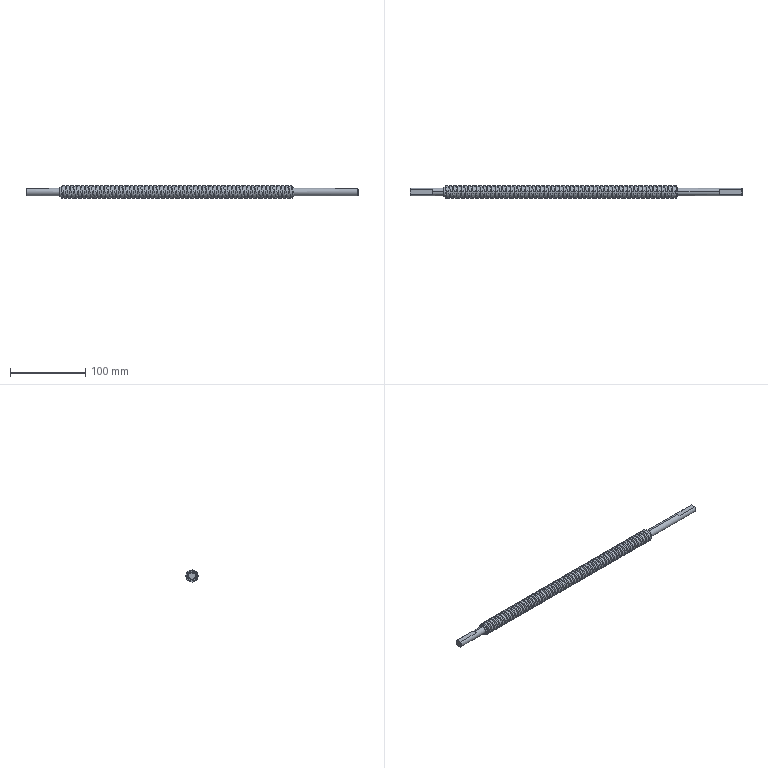Part | STEP file | 1605 ball screw | 1 solid | 148 faces | box 440 x 16 x 16 mm | volume 67458 mm3 | cylinder 132 | plane 12 | cone 3 | spline 1 | commonest cylinder face diameters 16 x124 10 x4 13 x4